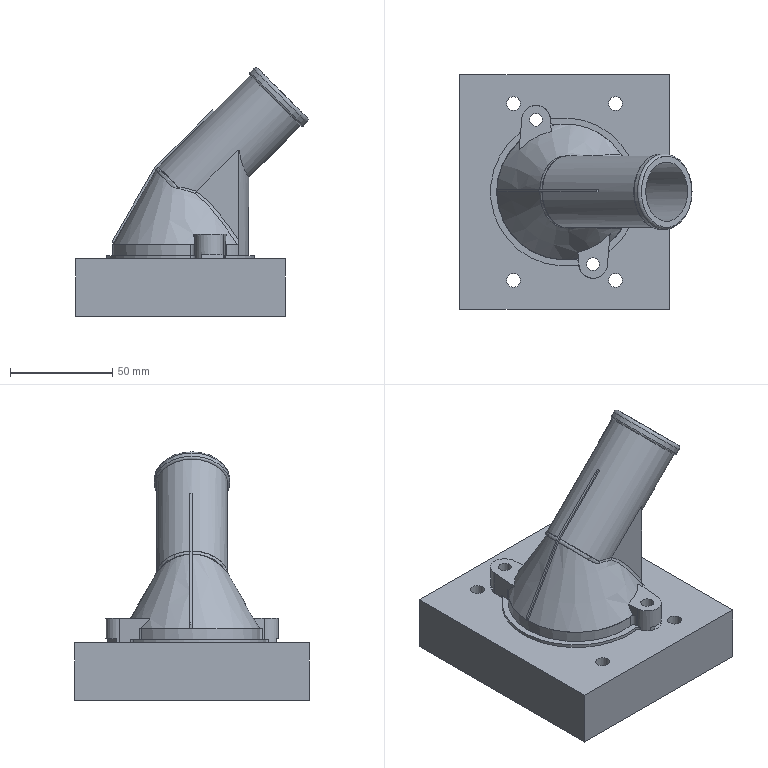NC program | NX | posted by the shop | part box 113.679 x 114.654 x 121.568 mm
Lines 24445 to 25302 of 160120:
24444 * - OPERATION: 等高混合 - TOOL: T5 J-D10R0.5
24445 TOOL CALL Z S8000
24446 M3
24447 CYCL DEF 32.0 TOLERANCE
24448 CYCL DEF 32.1 T0.006
24449 CYCL DEF 32.2 HSC-MODE:0
24450 PLANE SPATIAL SPA-45. SPB+0.0 SPC-90. TURN FMAX SEQ-
24451 L X-2.0005 Y-34.1938 FMAX
24452 L Z171.5197 FMAX
24453 L Z97.5563 FMAX
24454 L Y-34.4655 F250.
24455 CC X-.0005 Y-34.4655
24456 C X-.0005 Y-36.4655 DR+
24457 CC X-.0005 Y-26.9682
24458 C X9.2748 Y-24.9267 DR+ F2500.
24459 CC X.001 Y-26.968
24460 C X-5.4413 Y-19.1865 DR+
24461 CC X-.019 Y-26.9568
24462 C X-9.061 Y-24.1245 DR+
24463 CC X.0018 Y-26.9678
24464 C X-2.3798 Y-36.1627 DR+
24465 CC X-.0005 Y-26.9682
24466 C X-.0005 Y-36.4655 DR+
24467 L Y-36.4659 Z97.3563
24468 CC X.0021 Y-26.9665
24469 C X-9.2835 Y-24.9622 DR-
24470 CC X.0044 Y-26.9738
24471 C X-1.9169 Y-17.6668 DR-
24472 CC X-.0009 Y-26.969
24473 C X1.5286 Y-36.3425 DR-
24474 CC X.0021 Y-26.9665
24475 C X-.0005 Y-36.4659 DR-
24476 L Y-36.4651 Z97.1563
24477 CC X.0011 Y-26.9665
24478 C X7.6999 Y-32.5299 DR+
24479 CC X-.0037 Y-26.97
24480 C X7.0017 Y-20.5527 DR+
24481 CC X.0009 Y-26.967
24482 C X-5.4413 Y-19.1865 DR+
24483 L X-5.5464 Y-19.2588
24484 CC X.0152 Y-26.9791
24485 C X-9.2835 Y-24.9622 DR+
24486 CC X.0011 Y-26.9665
24487 C X-.0005 Y-36.4651 DR+
24488 L Y-36.4686 Z96.9563
24489 CC X+0.0 Y-26.9686
24490 C X-9.3132 Y-28.8433 DR-
24491 L X-9.3113 Y-28.8321
24492 L X-9.3321 Y-28.7469
24493 L X-9.3726 Y-28.5021
24494 L X-9.3761 Y-28.4978
24495 CC X+0.0 Y-26.9686
24496 C X-9.3867 Y-28.4311 DR-
24497 L X-9.3877 Y-28.4062
24498 L X-9.4305 Y-28.1159
24499 L X-9.4635 Y-27.8004
24500 CC X-13.1362 Y-27.9031
24501 C X-9.486 Y-27.4848 DR+
24502 CC X+0.0 Y-26.9686
24503 C X-9.4882 Y-27.4413 DR-
24504 L X-9.4906 Y-27.2638
24505 L X-9.4979 Y-27.1695
24506 CC X-4.1304 Y-27.0299
24507 C X-9.4927 Y-26.7569 DR-
24508 CC X-6.8804 Y-26.6774
24509 C X-9.4762 Y-26.3731 DR-
24510 CC X-10.4058 Y-26.2641
24511 C X-9.4707 Y-26.2231 DR+
24512 CC X+0.0 Y-26.9686
24513 C X-9.1205 Y-24.3102 DR-
24514 L X-9.1129 Y-24.3018
24515 L X-9.0809 Y-24.193
24516 CC X-4.9494 Y-25.3485
24517 C X-8.9622 Y-23.8313 DR-
24518 CC X-3.7836 Y-25.5358
24519 C X-8.8044 Y-23.4111 DR-
24520 L X-8.7419 Y-23.2605
24521 CC X-5.6947 Y-24.443
24522 C X-8.6158 Y-22.9764 DR-
24523 L X-8.5527 Y-22.8434
24524 CC X-4.0156 Y-24.9206
24525 C X-8.3627 Y-22.4705 DR-
24526 L X-8.3004 Y-22.3561
24527 CC X-4.3618 Y-24.4354
24528 C X-8.1107 Y-22.0308 DR-
24529 CC X-2.5469 Y-25.3283
24530 C X-7.8589 Y-21.639 DR-
24531 L X-7.7954 Y-21.5461
24532 CC X-3.3317 Y-24.544
24533 C X-7.543 Y-21.2007 DR-
24534 CC X-.0735 Y-26.8883
24535 C X-4.9497 Y-18.8655 DR-
24536 CC X-2.2686 Y-23.059
24537 C X-4.5883 Y-18.6553 DR-
24538 CC X-.5236 Y-25.9087
24539 C X-3.9654 Y-18.3399 DR-
24540 L X-3.6406 Y-18.1989
24541 L X-3.6008 Y-18.1825
24542 CC X-.1906 Y-26.4741
24543 C X-3.1876 Y-18.0244 DR-
24544 L X-2.76 Y-17.883
24545 L X-2.7056 Y-17.867
24546 CC X-.6756 Y-24.3584
24547 C X-2.1077 Y-17.7095 DR-
24548 CC X-.2639 Y-25.5223
24549 C X-1.2172 Y-17.5517 DR-
24550 CC X.0003 Y-26.7938
24551 C X1.2209 Y-17.5521 DR-
24552 CC X.1698 Y-26.0468
24553 C X2.1094 Y-17.71 DR-
24554 CC X.2842 Y-25.8515
24555 C X2.7073 Y-17.8675 DR-
24556 CC X1.077 Y-23.6757
24557 C X3.1915 Y-18.0257 DR-
24558 CC X.9332 Y-24.5336
24559 C X3.6019 Y-18.183 DR-
24560 CC X.4571 Y-26.0172
24561 C X4.5906 Y-18.6566 DR-
24562 CC X2.4001 Y-22.8347
24563 C X4.952 Y-18.867 DR-
24564 CC X.7925 Y-25.8113
24565 C X5.7231 Y-19.3915 DR-
24566 CC X.1349 Y-26.8325
24567 C X7.541 Y-21.1981 DR-
24568 CC X2.8799 Y-24.8807
24569 C X7.8452 Y-21.6198 DR-
24570 L X7.8483 Y-21.6236
24571 CC X2.9993 Y-25.031
24572 C X8.0984 Y-22.0107 DR-
24573 CC X2.9333 Y-25.2799
24574 C X8.3509 Y-22.4486 DR-
24575 L X8.5064 Y-22.7456
24576 L X8.54 Y-22.8164
24577 L X8.6029 Y-22.9487
24578 CC X5.1954 Y-24.645
24579 C X8.7282 Y-23.2278 DR-
24580 L X8.7922 Y-23.3816
24581 CC X5.0004 Y-25.0492
24582 C X8.9339 Y-23.7508 DR-
24583 CC X3.5546 Y-25.7909
24584 C X9.0913 Y-24.2276 DR-
24585 L X9.1307 Y-24.3601
24586 CC X.2535 Y-26.9171
24587 C X9.4016 Y-25.6304 DR-
24588 L X9.406 Y-25.6353
24589 CC X+0.0 Y-26.9686
24590 C X-.0005 Y-36.4686 DR-
24591 L Z96.7563
24592 CC X+0.0 Y-26.9686
24593 C X9.406 Y-25.6353 DR+
24594 L X9.4016 Y-25.6304
24595 CC X.2534 Y-26.9185
24596 C X9.1301 Y-24.3587 DR+
24597 L X9.0908 Y-24.2258
24598 CC X3.5547 Y-25.7924
24599 C X8.9331 Y-23.749 DR+
24600 CC X5.0005 Y-25.0511
24601 C X8.7912 Y-23.3804 DR+
24602 L X8.7276 Y-23.2257
24603 CC X5.1959 Y-24.6477
24604 C X8.6015 Y-22.9456 DR+
24605 L X8.5386 Y-22.8134
24606 L X8.5064 Y-22.7456
24607 L X8.349 Y-22.4452
24608 CC X2.9314 Y-25.2769
24609 C X8.0972 Y-22.0084 DR+
24610 CC X3.0024 Y-25.0361
24611 C X7.8452 Y-21.6198 DR+
24612 CC X2.8789 Y-24.8798
24613 C X7.5404 Y-21.1971 DR+
24614 CC X.1352 Y-26.8327
24615 C X5.7231 Y-19.3915 DR+
24616 CC X.7913 Y-25.8107
24617 C X4.9499 Y-18.8655 DR+
24618 CC X2.395 Y-22.842
24619 C X4.5884 Y-18.6553 DR+
24620 CC X.458 Y-26.0177
24621 C X3.5998 Y-18.1822 DR+
24622 CC X.9262 Y-24.549
24623 C X3.1889 Y-18.0248 DR+
24624 CC X1.0747 Y-23.6754
24625 C X2.706 Y-17.867 DR+
24626 CC X.2846 Y-25.8523
24627 C X2.1061 Y-17.7092 DR+
24628 CC X.1696 Y-26.0471
24629 C X1.2178 Y-17.5517 DR+
24630 CC X-.0002 Y-26.794
24631 C X-1.2212 Y-17.5521 DR+
24632 CC X-.2628 Y-25.5223
24633 C X-2.1101 Y-17.7101 DR+
24634 CC X-.6779 Y-24.3595
24635 C X-2.7075 Y-17.8675 DR+
24636 L X-2.76 Y-17.883
24637 L X-3.1898 Y-18.0252
24638 CC X-.1912 Y-26.4729
24639 C X-3.6008 Y-18.1825 DR+
24640 L X-3.6406 Y-18.1989
24641 L X-3.9673 Y-18.3408
24642 CC X-.526 Y-25.9102
24643 C X-4.5897 Y-18.6559 DR+
24644 CC X-2.2671 Y-23.0581
24645 C X-4.9503 Y-18.8659 DR+
24646 CC X-.0739 Y-26.8887
24647 C X-7.5452 Y-21.2033 DR+
24648 CC X-3.3307 Y-24.543
24649 C X-7.7968 Y-21.548 DR+
24650 L X-7.8596 Y-21.6401
24651 CC X-2.5255 Y-25.3461
24652 C X-8.1119 Y-22.0325 DR+
24653 CC X-4.3618 Y-24.4366
24654 C X-8.3009 Y-22.3566 DR+
24655 L X-8.3647 Y-22.4742
24656 CC X-4.0158 Y-24.9214
24657 C X-8.5527 Y-22.8434 DR+
24658 L X-8.6165 Y-22.977
24659 CC X-5.6954 Y-24.4445
24660 C X-8.7438 Y-23.2641 DR+
24661 L X-8.806 Y-23.4156
24662 CC X-5.1642 Y-25.0229
24663 C X-8.9631 Y-23.8335 DR+
24664 CC X-4.9502 Y-25.3541
24665 C X-9.0831 Y-24.1987 DR+
24666 L X-9.1129 Y-24.3018
24667 L X-9.1205 Y-24.3102
24668 CC X+0.0 Y-26.9686
24669 C X-9.4707 Y-26.2231 DR+
24670 CC X-10.4059 Y-26.2641
24671 C X-9.4762 Y-26.3731 DR-
24672 CC X-6.8804 Y-26.6774
24673 C X-9.4927 Y-26.7569 DR+
24674 CC X-4.1306 Y-27.0299
24675 C X-9.4979 Y-27.1695 DR+
24676 L X-9.4906 Y-27.2638
24677 L X-9.4882 Y-27.4413
24678 CC X+0.0 Y-26.9686
24679 C X-9.486 Y-27.4848 DR+
24680 CC X-13.1361 Y-27.9031
24681 C X-9.4635 Y-27.8004 DR-
24682 L X-9.4305 Y-28.1159
24683 L X-9.3877 Y-28.4062
24684 L X-9.3867 Y-28.4311
24685 CC X+0.0 Y-26.9686
24686 C X-9.3761 Y-28.4978 DR+
24687 L X-9.3726 Y-28.502
24688 L X-9.3321 Y-28.7469
24689 L X-9.3113 Y-28.8321
24690 L X-9.3132 Y-28.8433
24691 CC X+0.0 Y-26.9686
24692 C X-.0005 Y-36.4686 DR+
24693 L Z96.5563
24694 CC X+0.0 Y-26.9686
24695 C X-9.3132 Y-28.8433 DR-
24696 L X-9.3113 Y-28.8321
24697 L X-9.3321 Y-28.7469
24698 L X-9.3726 Y-28.502
24699 L X-9.3761 Y-28.4978
24700 CC X+0.0 Y-26.9686
24701 C X-9.3867 Y-28.4311 DR-
24702 L X-9.3877 Y-28.4062
24703 L X-9.4305 Y-28.1159
24704 L X-9.4635 Y-27.8004
24705 L X-9.4711 Y-27.6456
24706 L X-9.486 Y-27.4848
24707 CC X+0.0 Y-26.9686
24708 C X-9.4882 Y-27.4413 DR-
24709 L X-9.4906 Y-27.2638
24710 L X-9.4979 Y-27.1695
24711 CC X-4.1309 Y-27.0299
24712 C X-9.4927 Y-26.7569 DR-
24713 CC X-6.8804 Y-26.6774
24714 C X-9.4762 Y-26.3731 DR-
24715 CC X-10.4059 Y-26.2641
24716 C X-9.4707 Y-26.2231 DR+
24717 CC X+0.0 Y-26.9686
24718 C X-9.1205 Y-24.3102 DR-
24719 L X-9.1129 Y-24.3018
24720 L X-9.0809 Y-24.193
24721 CC X-4.9479 Y-25.3489
24722 C X-8.9622 Y-23.8313 DR-
24723 CC X-5.1487 Y-25.0233
24724 C X-8.8044 Y-23.4111 DR-
24725 L X-8.7419 Y-23.2605
24726 CC X-5.695 Y-24.4429
24727 C X-8.6158 Y-22.9764 DR-
24728 L X-8.5527 Y-22.8434
24729 CC X-4.0153 Y-24.9208
24730 C X-8.3627 Y-22.4705 DR-
24731 L X-8.3004 Y-22.3561
24732 CC X-4.3609 Y-24.4359
24733 C X-8.1107 Y-22.0308 DR-
24734 CC X-2.5003 Y-25.3583
24735 C X-7.8589 Y-21.639 DR-
24736 L X-7.7954 Y-21.5461
24737 CC X-3.3313 Y-24.5442
24738 C X-7.543 Y-21.2007 DR-
24739 CC X-.0735 Y-26.8883
24740 C X-4.9497 Y-18.8655 DR-
24741 CC X-2.2686 Y-23.0591
24742 C X-4.5883 Y-18.6553 DR-
24743 CC X-.5235 Y-25.909
24744 C X-3.9654 Y-18.3399 DR-
24745 L X-3.6406 Y-18.1989
24746 L X-3.6008 Y-18.1825
24747 CC X-.1916 Y-26.4716
24748 C X-3.1876 Y-18.0244 DR-
24749 L X-2.76 Y-17.883
24750 L X-2.7056 Y-17.867
24751 CC X-.6754 Y-24.3592
24752 C X-2.1077 Y-17.7095 DR-
24753 CC X-.2638 Y-25.5228
24754 C X-1.2172 Y-17.5517 DR-
24755 CC X.0003 Y-26.794
24756 C X1.2209 Y-17.5521 DR-
24757 CC X.1697 Y-26.0474
24758 C X2.1094 Y-17.71 DR-
24759 CC X.2838 Y-25.8529
24760 C X2.7073 Y-17.8675 DR-
24761 CC X1.0768 Y-23.6765
24762 C X3.1915 Y-18.0257 DR-
24763 CC X.921 Y-24.5653
24764 C X3.6019 Y-18.183 DR-
24765 CC X.457 Y-26.0173
24766 C X4.5906 Y-18.6566 DR-
24767 CC X2.3911 Y-22.8502
24768 C X4.952 Y-18.867 DR-
24769 CC X.7925 Y-25.8114
24770 C X5.7231 Y-19.3915 DR-
24771 CC X.1349 Y-26.8325
24772 C X7.541 Y-21.1981 DR-
24773 CC X2.8796 Y-24.8809
24774 C X7.8452 Y-21.6198 DR-
24775 L X7.8483 Y-21.6237
24776 CC X2.9992 Y-25.0311
24777 C X8.0984 Y-22.0107 DR-
24778 CC X2.933 Y-25.28
24779 C X8.3509 Y-22.4486 DR-
24780 L X8.5064 Y-22.7456
24781 L X8.54 Y-22.8164
24782 L X8.6029 Y-22.9487
24783 CC X5.194 Y-24.6457
24784 C X8.7282 Y-23.2279 DR-
24785 L X8.7922 Y-23.3816
24786 CC X4.9994 Y-25.0495
24787 C X8.9339 Y-23.7508 DR-
24788 CC X3.554 Y-25.7911
24789 C X9.0913 Y-24.2276 DR-
24790 L X9.1307 Y-24.3601
24791 CC X.2529 Y-26.9172
24792 C X9.4016 Y-25.6304 DR-
24793 L X9.406 Y-25.6353
24794 CC X+0.0 Y-26.9686
24795 C X-.0005 Y-36.4686 DR-
24796 L Z96.3563
24797 CC X+0.0 Y-26.9686
24798 C X9.406 Y-25.6353 DR+
24799 L X9.4016 Y-25.6304
24800 CC X.2528 Y-26.9186
24801 C X9.1301 Y-24.3587 DR+
24802 L X9.0908 Y-24.2258
24803 CC X3.5541 Y-25.7926
24804 C X8.9331 Y-23.749 DR+
24805 CC X4.9996 Y-25.0515
24806 C X8.7912 Y-23.3804 DR+
24807 L X8.7276 Y-23.2257
24808 CC X5.1945 Y-24.6484
24809 C X8.6015 Y-22.9456 DR+
24810 L X8.5386 Y-22.8134
24811 L X8.5064 Y-22.7456
24812 L X8.349 Y-22.4452
24813 CC X2.9311 Y-25.277
24814 C X8.0972 Y-22.0084 DR+
24815 CC X3.0023 Y-25.0362
24816 C X7.8452 Y-21.6198 DR+
24817 CC X2.8787 Y-24.88
24818 C X7.5404 Y-21.1971 DR+
24819 CC X.1352 Y-26.8326
24820 C X5.7231 Y-19.3915 DR+
24821 CC X.7913 Y-25.8108
24822 C X4.9499 Y-18.8655 DR+
24823 CC X2.3859 Y-22.8576
24824 C X4.5884 Y-18.6553 DR+
24825 CC X.4579 Y-26.0178
24826 C X3.5998 Y-18.1822 DR+
24827 CC X.914 Y-24.5808
24828 C X3.1889 Y-18.0248 DR+
24829 CC X1.0744 Y-23.6762
24830 C X2.706 Y-17.867 DR+
24831 CC X.2843 Y-25.8537
24832 C X2.1061 Y-17.7092 DR+
24833 CC X.1695 Y-26.0476
24834 C X1.2178 Y-17.5517 DR+
24835 CC X-.0002 Y-26.7942
24836 C X-1.2212 Y-17.5521 DR+
24837 CC X-.2627 Y-25.5228
24838 C X-2.1101 Y-17.7101 DR+
24839 CC X-.6777 Y-24.3603
24840 C X-2.7075 Y-17.8675 DR+
24841 L X-2.76 Y-17.883
24842 L X-3.1898 Y-18.0252
24843 CC X-.2518 Y-26.3145
24844 C X-3.6008 Y-18.1825 DR+
24845 L X-3.9171 Y-18.3168
24846 L X-3.9673 Y-18.3408
24847 CC X-.5259 Y-25.9104
24848 C X-4.5897 Y-18.6559 DR+
24849 CC X-2.2671 Y-23.0582
24850 C X-4.9503 Y-18.8659 DR+
24851 CC X-.0739 Y-26.8887
24852 C X-7.5451 Y-21.2033 DR+
24853 CC X-3.3304 Y-24.5432
24854 C X-7.7968 Y-21.548 DR+
24855 L X-7.8596 Y-21.6401
24856 CC X-2.4785 Y-25.3763
24857 C X-8.1119 Y-22.0326 DR+
24858 CC X-4.361 Y-24.4371
24859 C X-8.3009 Y-22.3566 DR+
24860 L X-8.3647 Y-22.4742
24861 CC X-4.0155 Y-24.9216
24862 C X-8.5527 Y-22.8434 DR+
24863 L X-8.6165 Y-22.977
24864 CC X-5.6956 Y-24.4443
24865 C X-8.7438 Y-23.2641 DR+
24866 L X-8.806 Y-23.4156
24867 CC X-5.1368 Y-25.0332
24868 C X-8.9631 Y-23.8335 DR+
24869 CC X-4.9486 Y-25.3545
24870 C X-9.0831 Y-24.1987 DR+
24871 L X-9.1129 Y-24.3018
24872 L X-9.1205 Y-24.3102
24873 CC X+0.0 Y-26.9686
24874 C X-9.4707 Y-26.2231 DR+
24875 CC X-10.406 Y-26.2641
24876 C X-9.4762 Y-26.3731 DR-
24877 CC X-6.8805 Y-26.6774
24878 C X-9.4927 Y-26.7569 DR+
24879 CC X-4.1311 Y-27.0299
24880 C X-9.4979 Y-27.1695 DR+
24881 L X-9.4906 Y-27.2638
24882 L X-9.4882 Y-27.4413
24883 CC X+0.0 Y-26.9686
24884 C X-9.486 Y-27.4848 DR+
24885 CC X-13.136 Y-27.9031
24886 C X-9.4635 Y-27.8004 DR-
24887 L X-9.4305 Y-28.1159
24888 L X-9.3877 Y-28.4062
24889 L X-9.3867 Y-28.4311
24890 CC X+0.0 Y-26.9686
24891 C X-9.3761 Y-28.4978 DR+
24892 L X-9.3726 Y-28.502
24893 L X-9.3321 Y-28.7469
24894 L X-9.3113 Y-28.8321
24895 L X-9.3132 Y-28.8433
24896 CC X+0.0 Y-26.9686
24897 C X-.0005 Y-36.4686 DR+
24898 L Z96.1563
24899 CC X+0.0 Y-26.9686
24900 C X-9.3132 Y-28.8433 DR-
24901 L X-9.3113 Y-28.8321
24902 L X-9.3321 Y-28.7469
24903 L X-9.3726 Y-28.502
24904 L X-9.3761 Y-28.4978
24905 CC X+0.0 Y-26.9686
24906 C X-9.3867 Y-28.4311 DR-
24907 L X-9.3877 Y-28.4062
24908 L X-9.4305 Y-28.1159
24909 L X-9.4635 Y-27.8004
24910 CC X-13.1359 Y-27.9031
24911 C X-9.486 Y-27.4848 DR+
24912 CC X+0.0 Y-26.9686
24913 C X-9.4882 Y-27.4413 DR-
24914 L X-9.4906 Y-27.2638
24915 L X-9.4979 Y-27.1695
24916 CC X-4.1313 Y-27.0299
24917 C X-9.4927 Y-26.757 DR-
24918 CC X-6.8805 Y-26.6774
24919 C X-9.4762 Y-26.3731 DR-
24920 CC X-10.4061 Y-26.2641
24921 C X-9.4707 Y-26.2231 DR+
24922 CC X+0.0 Y-26.9686
24923 C X-9.1205 Y-24.3102 DR-
24924 L X-9.1129 Y-24.3018
24925 L X-9.0809 Y-24.193
24926 CC X-4.9464 Y-25.3494
24927 C X-8.9622 Y-23.8313 DR-
24928 CC X-5.1211 Y-25.0336
24929 C X-8.8044 Y-23.4111 DR-
24930 L X-8.7419 Y-23.2605
24931 CC X-5.6952 Y-24.4428
24932 C X-8.6158 Y-22.9764 DR-
24933 L X-8.5527 Y-22.8434
24934 CC X-4.0149 Y-24.921
24935 C X-8.3627 Y-22.4705 DR-
24936 L X-8.3004 Y-22.3561
24937 CC X-4.3601 Y-24.4364
24938 C X-8.1107 Y-22.0308 DR-
24939 CC X-2.4529 Y-25.3887
24940 C X-7.8589 Y-21.639 DR-
24941 L X-7.7954 Y-21.5461
24942 CC X-3.331 Y-24.5445
24943 C X-7.543 Y-21.2008 DR-
24944 CC X-.0735 Y-26.8882
24945 C X-4.9497 Y-18.8655 DR-
24946 CC X-2.2685 Y-23.0592
24947 C X-4.5883 Y-18.6553 DR-
24948 CC X-.5233 Y-25.9092
24949 C X-3.9654 Y-18.3399 DR-
24950 L X-3.9171 Y-18.3168
24951 L X-3.6008 Y-18.1825
24952 CC X-.2518 Y-26.3142
24953 C X-3.1876 Y-18.0244 DR-
24954 L X-2.76 Y-17.883
24955 L X-2.7056 Y-17.867
24956 CC X-.6751 Y-24.3601
24957 C X-2.1077 Y-17.7095 DR-
24958 CC X-.2638 Y-25.5233
24959 C X-1.2172 Y-17.5517 DR-
24960 CC X.0003 Y-26.7942
24961 C X1.2209 Y-17.5521 DR-
24962 CC X.1696 Y-26.048
24963 C X2.1094 Y-17.71 DR-
24964 CC X.2835 Y-25.8542
24965 C X2.7073 Y-17.8675 DR-
24966 CC X1.0765 Y-23.6773
24967 C X3.1915 Y-18.0257 DR-
24968 CC X.9088 Y-24.5972
24969 C X3.6019 Y-18.183 DR-
24970 CC X.457 Y-26.0174
24971 C X4.5906 Y-18.6566 DR-
24972 CC X2.382 Y-22.8658
24973 C X4.952 Y-18.867 DR-
24974 CC X.7924 Y-25.8116
24975 C X5.7231 Y-19.3915 DR-
24976 CC X.135 Y-26.8324
24977 C X7.541 Y-21.1981 DR-
24978 CC X2.8793 Y-24.8811
24979 C X7.8452 Y-21.6198 DR-
24980 L X7.8483 Y-21.6237
24981 CC X2.9991 Y-25.0311
24982 C X8.0984 Y-22.0107 DR-
24983 CC X2.9328 Y-25.2801
24984 C X8.3509 Y-22.4486 DR-
24985 L X8.5064 Y-22.7456
24986 L X8.54 Y-22.8164
24987 L X8.6029 Y-22.9487
24988 CC X5.1927 Y-24.6463
24989 C X8.7282 Y-23.2279 DR-
24990 L X8.7922 Y-23.3816
24991 CC X4.9985 Y-25.0499
24992 C X8.9339 Y-23.7508 DR-
24993 CC X3.5534 Y-25.7913
24994 C X9.0913 Y-24.2276 DR-
24995 L X9.1307 Y-24.3601
24996 CC X.2524 Y-26.9173
24997 C X9.4016 Y-25.6304 DR-
24998 L X9.406 Y-25.6353
24999 CC X+0.0 Y-26.9686
25000 C X-.0005 Y-36.4686 DR-
25001 L Z95.9563
25002 CC X+0.0 Y-26.9686
25003 C X9.406 Y-25.6353 DR+
25004 L X9.4016 Y-25.6304
25005 CC X.2523 Y-26.9187
25006 C X9.1301 Y-24.3587 DR+
25007 L X9.0908 Y-24.2258
25008 CC X3.5535 Y-25.7928
25009 C X8.9331 Y-23.749 DR+
25010 CC X4.9987 Y-25.0518
25011 C X8.7912 Y-23.3804 DR+
25012 L X8.7276 Y-23.2257
25013 CC X5.1932 Y-24.649
25014 C X8.6015 Y-22.9457 DR+
25015 L X8.5386 Y-22.8134
25016 L X8.5064 Y-22.7456
25017 L X8.349 Y-22.4452
25018 CC X2.9309 Y-25.2772
25019 C X8.0972 Y-22.0084 DR+
25020 CC X3.0022 Y-25.0362
25021 C X7.8452 Y-21.6198 DR+
25022 CC X2.8784 Y-24.8801
25023 C X7.5404 Y-21.1971 DR+
25024 CC X.1353 Y-26.8326
25025 C X5.7231 Y-19.3915 DR+
25026 CC X.7912 Y-25.8109
25027 C X4.9499 Y-18.8655 DR+
25028 CC X2.3768 Y-22.8733
25029 C X4.5884 Y-18.6553 DR+
25030 CC X.4579 Y-26.0178
25031 C X3.5998 Y-18.1822 DR+
25032 CC X.9017 Y-24.6129
25033 C X3.1889 Y-18.0248 DR+
25034 CC X1.0741 Y-23.6769
25035 C X2.706 Y-17.867 DR+
25036 CC X.2839 Y-25.8551
25037 C X2.1061 Y-17.7092 DR+
25038 CC X.1694 Y-26.0482
25039 C X1.2178 Y-17.5517 DR+
25040 CC X-.0002 Y-26.7944
25041 C X-1.2212 Y-17.5521 DR+
25042 CC X-.2626 Y-25.5234
25043 C X-2.1101 Y-17.7101 DR+
25044 CC X-.6774 Y-24.3612
25045 C X-2.7075 Y-17.8675 DR+
25046 L X-2.76 Y-17.883
25047 L X-3.1898 Y-18.0252
25048 CC X-.252 Y-26.314
25049 C X-3.6008 Y-18.1825 DR+
25050 L X-3.9171 Y-18.3168
25051 L X-3.9673 Y-18.3408
25052 CC X-.5258 Y-25.9107
25053 C X-4.5897 Y-18.6559 DR+
25054 CC X-2.267 Y-23.0583
25055 C X-4.9503 Y-18.8659 DR+
25056 CC X-.0739 Y-26.8887
25057 C X-7.5451 Y-21.2033 DR+
25058 CC X-3.3301 Y-24.5434
25059 C X-7.7968 Y-21.548 DR+
25060 L X-7.8596 Y-21.6401
25061 CC X-2.4308 Y-25.4069
25062 C X-8.1119 Y-22.0326 DR+
25063 CC X-4.3602 Y-24.4376
25064 C X-8.3009 Y-22.3566 DR+
25065 L X-8.3647 Y-22.4742
25066 CC X-4.0151 Y-24.9218
25067 C X-8.5527 Y-22.8434 DR+
25068 L X-8.6165 Y-22.977
25069 CC X-5.6959 Y-24.4442
25070 C X-8.7438 Y-23.2641 DR+
25071 L X-8.806 Y-23.4156
25072 CC X-5.1091 Y-25.0436
25073 C X-8.9631 Y-23.8336 DR+
25074 CC X-4.9471 Y-25.355
25075 C X-9.083 Y-24.1987 DR+
25076 L X-9.1129 Y-24.3018
25077 L X-9.1205 Y-24.3102
25078 CC X+0.0 Y-26.9686
25079 C X-9.4707 Y-26.2231 DR+
25080 CC X-10.4061 Y-26.2641
25081 C X-9.4762 Y-26.3731 DR-
25082 CC X-6.8806 Y-26.6774
25083 C X-9.4927 Y-26.757 DR+
25084 CC X-4.1315 Y-27.0299
25085 C X-9.4979 Y-27.1695 DR+
25086 L X-9.4906 Y-27.2638
25087 L X-9.4882 Y-27.4413
25088 CC X+0.0 Y-26.9686
25089 C X-9.486 Y-27.4848 DR+
25090 CC X-13.1358 Y-27.9031
25091 C X-9.4635 Y-27.8004 DR-
25092 L X-9.4305 Y-28.1159
25093 L X-9.3877 Y-28.4062
25094 L X-9.3867 Y-28.4311
25095 CC X+0.0 Y-26.9686
25096 C X-9.3761 Y-28.4978 DR+
25097 L X-9.3726 Y-28.502
25098 L X-9.3321 Y-28.7469
25099 L X-9.3113 Y-28.8321
25100 L X-9.3132 Y-28.8433
25101 CC X+0.0 Y-26.9686
25102 C X-.0005 Y-36.4686 DR+
25103 L Z95.7563
25104 CC X+0.0 Y-26.9686
25105 C X-9.3132 Y-28.8433 DR-
25106 L X-9.3113 Y-28.8321
25107 L X-9.3321 Y-28.7469
25108 L X-9.3726 Y-28.502
25109 L X-9.3761 Y-28.4978
25110 CC X+0.0 Y-26.9686
25111 C X-9.3867 Y-28.4311 DR-
25112 L X-9.3877 Y-28.4062
25113 L X-9.4305 Y-28.1159
25114 L X-9.4635 Y-27.8004
25115 CC X-13.1358 Y-27.9031
25116 C X-9.486 Y-27.4848 DR+
25117 CC X+0.0 Y-26.9686
25118 C X-9.4882 Y-27.4413 DR-
25119 L X-9.4906 Y-27.2638
25120 L X-9.4979 Y-27.1695
25121 CC X-4.1318 Y-27.0299
25122 C X-9.4927 Y-26.757 DR-
25123 CC X-6.8806 Y-26.6775
25124 C X-9.4762 Y-26.3731 DR-
25125 CC X-10.4062 Y-26.2641
25126 C X-9.4707 Y-26.2231 DR+
25127 CC X+0.0 Y-26.9686
25128 C X-9.1205 Y-24.3102 DR-
25129 L X-9.1129 Y-24.3018
25130 L X-9.0809 Y-24.1931
25131 CC X-4.9449 Y-25.3499
25132 C X-8.9622 Y-23.8313 DR-
25133 CC X-5.0932 Y-25.0441
25134 C X-8.8044 Y-23.4111 DR-
25135 L X-8.7419 Y-23.2605
25136 CC X-5.6954 Y-24.4427
25137 C X-8.6158 Y-22.9764 DR-
25138 L X-8.5527 Y-22.8434
25139 CC X-4.0145 Y-24.9212
25140 C X-8.3627 Y-22.4705 DR-
25141 L X-8.3004 Y-22.3561
25142 CC X-4.3593 Y-24.4369
25143 C X-8.1106 Y-22.0308 DR-
25144 CC X-2.4049 Y-25.4196
25145 C X-7.8589 Y-21.639 DR-
25146 L X-7.7954 Y-21.5461
25147 CC X-3.2938 Y-24.5716
25148 C X-7.543 Y-21.2008 DR-
25149 CC X-.0736 Y-26.8882
25150 C X-4.9497 Y-18.8655 DR-
25151 CC X-2.2685 Y-23.0593
25152 C X-4.5883 Y-18.6553 DR-
25153 CC X-.5232 Y-25.9095
25154 C X-3.9654 Y-18.3399 DR-
25155 L X-3.9171 Y-18.3168
25156 L X-3.6008 Y-18.1825
25157 CC X-.252 Y-26.3138
25158 C X-3.1876 Y-18.0244 DR-
25159 L X-2.76 Y-17.883
25160 L X-2.7056 Y-17.867
25161 CC X-.6749 Y-24.3609
25162 C X-2.1077 Y-17.7095 DR-
25163 CC X-.2637 Y-25.5238
25164 C X-1.2172 Y-17.5517 DR-
25165 CC X.0003 Y-26.7944
25166 C X1.2209 Y-17.5521 DR-
25167 CC X.1695 Y-26.0485
25168 C X2.1094 Y-17.71 DR-
25169 CC X.2831 Y-25.8556
25170 C X2.7073 Y-17.8675 DR-
25171 CC X1.0763 Y-23.678
25172 C X3.1915 Y-18.0257 DR-
25173 CC X.8964 Y-24.6294
25174 C X3.6019 Y-18.183 DR-
25175 CC X.457 Y-26.0175
25176 C X4.5906 Y-18.6566 DR-
25177 CC X2.3729 Y-22.8815
25178 C X4.952 Y-18.867 DR-
25179 CC X.7923 Y-25.8117
25180 C X5.7231 Y-19.3915 DR-
25181 CC X.135 Y-26.8324
25182 C X7.541 Y-21.1981 DR-
25183 CC X2.8791 Y-24.8813
25184 C X7.8452 Y-21.6198 DR-
25185 L X7.8483 Y-21.6237
25186 CC X2.999 Y-25.0312
25187 C X8.0984 Y-22.0107 DR-
25188 CC X2.9325 Y-25.2803
25189 C X8.3509 Y-22.4486 DR-
25190 L X8.5064 Y-22.7456
25191 L X8.54 Y-22.8164
25192 L X8.6029 Y-22.9487
25193 CC X5.1913 Y-24.6469
25194 C X8.7282 Y-23.2279 DR-
25195 L X8.7922 Y-23.3816
25196 CC X4.9976 Y-25.0502
25197 C X8.9339 Y-23.7508 DR-
25198 CC X3.5528 Y-25.7915
25199 C X9.0913 Y-24.2276 DR-
25200 L X9.1307 Y-24.3601
25201 CC X.2518 Y-26.9174
25202 C X9.4016 Y-25.6304 DR-
25203 L X9.406 Y-25.6353
25204 CC X+0.0 Y-26.9686
25205 C X-.0005 Y-36.4686 DR-
25206 L Z95.5563
25207 CC X+0.0 Y-26.9686
25208 C X9.406 Y-25.6353 DR+
25209 L X9.4016 Y-25.6304
25210 CC X.2517 Y-26.9188
25211 C X9.1301 Y-24.3587 DR+
25212 L X9.0908 Y-24.2258
25213 CC X3.5529 Y-25.793
25214 C X8.9331 Y-23.749 DR+
25215 CC X4.9978 Y-25.0522
25216 C X8.7912 Y-23.3804 DR+
25217 L X8.7276 Y-23.2257
25218 CC X5.1918 Y-24.6496
25219 C X8.6015 Y-22.9457 DR+
25220 L X8.5386 Y-22.8134
25221 L X8.5064 Y-22.7456
25222 L X8.349 Y-22.4452
25223 CC X2.9306 Y-25.2773
25224 C X8.0972 Y-22.0084 DR+
25225 CC X3.0021 Y-25.0363
25226 C X7.8452 Y-21.6198 DR+
25227 CC X2.8781 Y-24.8803
25228 C X7.5404 Y-21.1971 DR+
25229 CC X.1353 Y-26.8326
25230 C X5.7231 Y-19.3915 DR+
25231 CC X.7911 Y-25.8111
25232 C X4.9499 Y-18.8655 DR+
25233 CC X2.3676 Y-22.8891
25234 C X4.5884 Y-18.6553 DR+
25235 CC X.4578 Y-26.0179
25236 C X3.5998 Y-18.1822 DR+
25237 CC X.8893 Y-24.6453
25238 C X3.1888 Y-18.0248 DR+
25239 CC X1.0739 Y-23.6777
25240 C X2.706 Y-17.867 DR+
25241 CC X.2836 Y-25.8564
25242 C X2.1061 Y-17.7092 DR+
25243 CC X.1693 Y-26.0488
25244 C X1.2178 Y-17.5517 DR+
25245 CC X-.0002 Y-26.7946
25246 C X-1.2212 Y-17.5521 DR+
25247 CC X-.2625 Y-25.5239
25248 C X-2.1101 Y-17.7101 DR+
25249 CC X-.6772 Y-24.362
25250 C X-2.7075 Y-17.8675 DR+
25251 L X-2.76 Y-17.883
25252 L X-3.1898 Y-18.0252
25253 CC X-.2522 Y-26.3135
25254 C X-3.6008 Y-18.1825 DR+
25255 L X-3.9171 Y-18.3168
25256 L X-3.9673 Y-18.3408
25257 CC X-.5256 Y-25.9109
25258 C X-4.5897 Y-18.6559 DR+
25259 CC X-2.267 Y-23.0584
25260 C X-4.9503 Y-18.8659 DR+
25261 CC X-.0739 Y-26.8886
25262 C X-7.5451 Y-21.2033 DR+
25263 CC X-3.2929 Y-24.5706
25264 C X-7.7968 Y-21.548 DR+
25265 L X-7.8596 Y-21.6401
25266 CC X-2.3825 Y-25.438
25267 C X-8.1119 Y-22.0326 DR+
25268 CC X-4.3593 Y-24.438
25269 C X-8.3009 Y-22.3566 DR+
25270 L X-8.3647 Y-22.4742
25271 CC X-4.0147 Y-24.922
25272 C X-8.5527 Y-22.8434 DR+
25273 L X-8.6165 Y-22.977
25274 CC X-5.6961 Y-24.4441
25275 C X-8.7438 Y-23.2641 DR+
25276 L X-8.806 Y-23.4156
25277 CC X-5.0809 Y-25.0542
25278 C X-8.9631 Y-23.8336 DR+
25279 CC X-4.9456 Y-25.3554
25280 C X-9.083 Y-24.1987 DR+
25281 L X-9.1129 Y-24.3018
25282 L X-9.1205 Y-24.3102
25283 CC X+0.0 Y-26.9686
25284 C X-9.4707 Y-26.2231 DR+
25285 CC X-10.4063 Y-26.2641
25286 C X-9.4762 Y-26.3732 DR-
25287 CC X-6.8807 Y-26.6775
25288 C X-9.4927 Y-26.757 DR+
25289 CC X-4.132 Y-27.0299
25290 C X-9.4979 Y-27.1695 DR+
25291 L X-9.4906 Y-27.2638
25292 L X-9.4882 Y-27.4413
25293 CC X+0.0 Y-26.9686
25294 C X-9.486 Y-27.4848 DR+
25295 CC X-13.1357 Y-27.9031
25296 C X-9.4635 Y-27.8004 DR-
25297 L X-9.4305 Y-28.1159
25298 L X-9.3877 Y-28.4062
25299 L X-9.3867 Y-28.4311
25300 CC X+0.0 Y-26.9686
25301 C X-9.3761 Y-28.4978 DR+